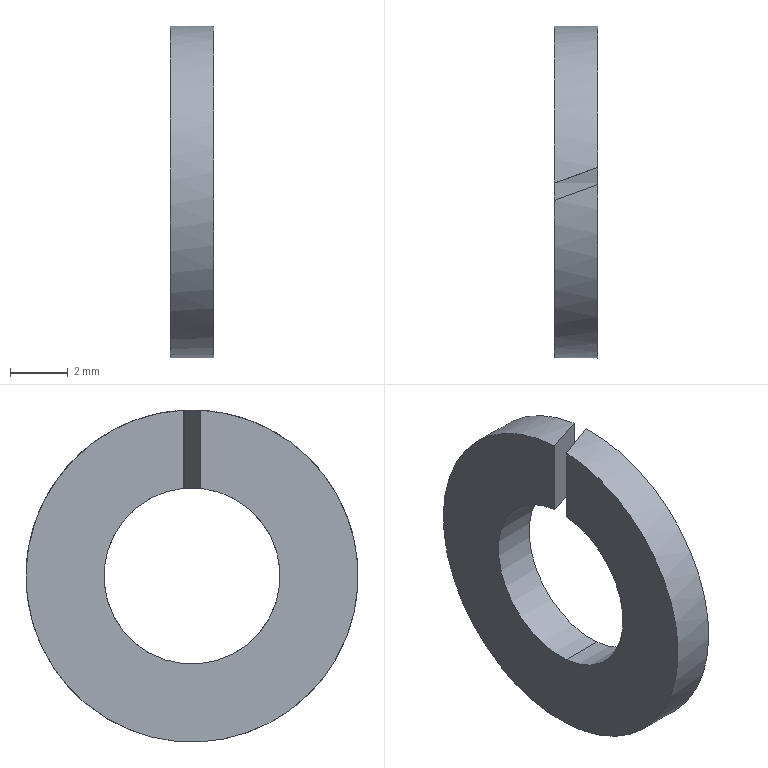Part | STEP file | KS B 1324 - No. 2 - 6 | 1 solid | 8 faces | box 1.5 x 11.5 x 11.5 mm | volume 109.527 mm3 | cylinder 4 | plane 4 | commonest cylinder face diameters 6.1 x2 11.5 x2
STEP:
#1=CARTESIAN_POINT('',(0.,0.,0.));
#2=DIRECTION('',(0.,0.,1.));
#3=DIRECTION('',(1.,0.,0.));
#4=AXIS2_PLACEMENT_3D('',#1,#2,#3);
#5=CARTESIAN_POINT('',(1.5,0.846,2.93));
#6=VERTEX_POINT('',#5);
#7=CARTESIAN_POINT('',(0.,0.3,3.035));
#8=VERTEX_POINT('',#7);
#9=CARTESIAN_POINT('',(1.5,0.846,2.93));
#10=CARTESIAN_POINT('',(1.009,0.6674,2.982));
#11=CARTESIAN_POINT('',(0.5081,0.4849,3.017));
#12=CARTESIAN_POINT('',(0.,0.3,3.035));
#13=(BOUNDED_CURVE()B_SPLINE_CURVE(3,(#9,#10,#11,#12),.UNSPECIFIED.,.F.,.F.)B_SPLINE_CURVE_WITH_KNOTS((4,4),(4.431,4.614),.PIECEWISE_BEZIER_KNOTS.)CURVE()GEOMETRIC_REPRESENTATION_ITEM()RATIONAL_B_SPLINE_CURVE((1.,0.9972,0.9972,1.))REPRESENTATION_ITEM(''));
#14=CARTESIAN_POINT('',(0.,0.,0.));
#15=DIRECTION('',(1.,0.,0.));
#16=DIRECTION('',(0.,-0.0895,-0.996));
#17=AXIS2_PLACEMENT_3D('',#14,#15,#16);
#18=CYLINDRICAL_SURFACE('',#17,3.05);
#19=CARTESIAN_POINT('',(2.95,1.5));
#20=CARTESIAN_POINT('',(2.953,1.478));
#21=CARTESIAN_POINT('',(2.958,1.433));
#22=CARTESIAN_POINT('',(2.967,1.366));
#23=CARTESIAN_POINT('',(2.975,1.299));
#24=CARTESIAN_POINT('',(2.983,1.232));
#25=CARTESIAN_POINT('',(2.992,1.164));
#26=CARTESIAN_POINT('',(3.,1.097));
#27=CARTESIAN_POINT('',(3.008,1.029));
#28=CARTESIAN_POINT('',(3.017,0.9611));
#29=CARTESIAN_POINT('',(3.025,0.893));
#30=CARTESIAN_POINT('',(3.033,0.8249));
#31=CARTESIAN_POINT('',(3.041,0.7566));
#32=CARTESIAN_POINT('',(3.05,0.6882));
#33=CARTESIAN_POINT('',(3.058,0.6197));
#34=CARTESIAN_POINT('',(3.066,0.5512));
#35=CARTESIAN_POINT('',(3.075,0.4825));
#36=CARTESIAN_POINT('',(3.083,0.4138));
#37=CARTESIAN_POINT('',(3.091,0.3449));
#38=CARTESIAN_POINT('',(3.1,0.2761));
#39=CARTESIAN_POINT('',(3.108,0.2071));
#40=CARTESIAN_POINT('',(3.116,0.1381));
#41=CARTESIAN_POINT('',(3.124,0.06908));
#42=CARTESIAN_POINT('',(3.13,0.02303));
#43=CARTESIAN_POINT('',(3.133,0.));
#44=B_SPLINE_CURVE_WITH_KNOTS('',3,(#19,#20,#21,#22,#23,#24,#25,#26,#27,#28,#29,#30,#31,#32,#33,#34,#35,#36,#37,#38,#39,#40,#41,#42,#43),.UNSPECIFIED.,.F.,.F.,(4,1,1,1,1,1,1,1,1,1,1,1,1,1,1,1,1,1,1,1,1,1,4),(4.431,4.44,4.448,4.456,4.465,4.473,4.481,4.489,4.498,4.506,4.514,4.523,4.531,4.539,4.547,4.556,4.564,4.572,4.581,4.589,4.597,4.606,4.614),.QUASI_UNIFORM_KNOTS.);
#45=(GEOMETRIC_REPRESENTATION_CONTEXT(2)PARAMETRIC_REPRESENTATION_CONTEXT()REPRESENTATION_CONTEXT('',''));
#46=DEFINITIONAL_REPRESENTATION('',(#44),#45);
#47=PCURVE('',#18,#46);
#48=CARTESIAN_POINT('',(0.,0.3,0.));
#49=DIRECTION('',(-0.342,0.9397,0.));
#50=DIRECTION('',(0.,0.,1.));
#51=AXIS2_PLACEMENT_3D('',#48,#49,#50);
#52=PLANE('',#51);
#53=CARTESIAN_POINT('',(2.93,1.596));
#54=CARTESIAN_POINT('',(2.982,1.074));
#55=CARTESIAN_POINT('',(3.017,0.5407));
#56=CARTESIAN_POINT('',(3.035,0.));
#57=(BOUNDED_CURVE()B_SPLINE_CURVE(3,(#53,#54,#55,#56),.UNSPECIFIED.,.F.,.F.)B_SPLINE_CURVE_WITH_KNOTS((4,4),(4.431,4.614),.PIECEWISE_BEZIER_KNOTS.)CURVE()GEOMETRIC_REPRESENTATION_ITEM()RATIONAL_B_SPLINE_CURVE((1.,0.9972,0.9972,1.))REPRESENTATION_ITEM(''));
#58=(GEOMETRIC_REPRESENTATION_CONTEXT(2)PARAMETRIC_REPRESENTATION_CONTEXT()REPRESENTATION_CONTEXT('',''));
#59=DEFINITIONAL_REPRESENTATION('',(#57),#58);
#60=PCURVE('',#52,#59);
#61=SURFACE_CURVE('',#13,(#47,#60),.PCURVE_S1.);
#62=EDGE_CURVE('',#6,#8,#61,.T.);
#63=ORIENTED_EDGE('',*,*,#62,.F.);
#64=CARTESIAN_POINT('',(1.5,-0.273,-3.038));
#65=VERTEX_POINT('',#64);
#66=CARTESIAN_POINT('',(1.5,0.,0.));
#67=DIRECTION('',(-1.,0.,0.));
#68=DIRECTION('',(0.,-1.,0.));
#69=AXIS2_PLACEMENT_3D('',#66,#67,#68);
#70=CIRCLE('',#69,3.05);
#71=CARTESIAN_POINT('',(4.802,1.5));
#72=DIRECTION('',(-1.,0.));
#73=VECTOR('',#72,1.);
#74=LINE('',#71,#73);
#75=(GEOMETRIC_REPRESENTATION_CONTEXT(2)PARAMETRIC_REPRESENTATION_CONTEXT()REPRESENTATION_CONTEXT('',''));
#76=DEFINITIONAL_REPRESENTATION('',(#74),#75);
#77=PCURVE('',#18,#76);
#78=CARTESIAN_POINT('',(1.5,0.,0.));
#79=DIRECTION('',(-1.,0.,0.));
#80=DIRECTION('',(0.,0.,1.));
#81=AXIS2_PLACEMENT_3D('',#78,#79,#80);
#82=PLANE('',#81);
#83=CARTESIAN_POINT('',(0.,0.));
#84=DIRECTION('',(0.,-1.));
#85=AXIS2_PLACEMENT_2D('',#83,#84);
#86=CIRCLE('',#85,3.05);
#87=(GEOMETRIC_REPRESENTATION_CONTEXT(2)PARAMETRIC_REPRESENTATION_CONTEXT()REPRESENTATION_CONTEXT('',''));
#88=DEFINITIONAL_REPRESENTATION('',(#86),#87);
#89=PCURVE('',#82,#88);
#90=SURFACE_CURVE('',#70,(#77,#89),.PCURVE_S1.);
#91=EDGE_CURVE('',#6,#65,#90,.T.);
#92=ORIENTED_EDGE('',*,*,#91,.T.);
#93=CARTESIAN_POINT('',(0.,-0.273,-3.038));
#94=VERTEX_POINT('',#93);
#95=CARTESIAN_POINT('',(0.,-0.273,-3.038));
#96=DIRECTION('',(1.,0.,0.));
#97=VECTOR('',#96,1.);
#98=LINE('',#95,#97);
#99=CARTESIAN_POINT('',(0.,0.));
#100=DIRECTION('',(0.,1.));
#101=VECTOR('',#100,1.);
#102=LINE('',#99,#101);
#103=(GEOMETRIC_REPRESENTATION_CONTEXT(2)PARAMETRIC_REPRESENTATION_CONTEXT()REPRESENTATION_CONTEXT('',''));
#104=DEFINITIONAL_REPRESENTATION('',(#102),#103);
#105=PCURVE('',#18,#104);
#106=CARTESIAN_POINT('',(0.,0.,0.));
#107=DIRECTION('',(1.,0.,0.));
#108=DIRECTION('',(0.,-0.0895,-0.996));
#109=AXIS2_PLACEMENT_3D('',#106,#107,#108);
#110=CYLINDRICAL_SURFACE('',#109,3.05);
#111=CARTESIAN_POINT('',(6.283,0.));
#112=DIRECTION('',(0.,1.));
#113=VECTOR('',#112,1.);
#114=LINE('',#111,#113);
#115=(GEOMETRIC_REPRESENTATION_CONTEXT(2)PARAMETRIC_REPRESENTATION_CONTEXT()REPRESENTATION_CONTEXT('',''));
#116=DEFINITIONAL_REPRESENTATION('',(#114),#115);
#117=PCURVE('',#110,#116);
#118=SURFACE_CURVE('',#98,(#105,#117),.PCURVE_S1.);
#119=EDGE_CURVE('',#94,#65,#118,.T.);
#120=ORIENTED_EDGE('',*,*,#119,.F.);
#121=CARTESIAN_POINT('',(0.,0.,0.));
#122=DIRECTION('',(1.,0.,0.));
#123=DIRECTION('',(0.,-1.,0.));
#124=AXIS2_PLACEMENT_3D('',#121,#122,#123);
#125=CIRCLE('',#124,3.05);
#126=CARTESIAN_POINT('',(-1.481,0.));
#127=DIRECTION('',(1.,0.));
#128=VECTOR('',#127,1.);
#129=LINE('',#126,#128);
#130=(GEOMETRIC_REPRESENTATION_CONTEXT(2)PARAMETRIC_REPRESENTATION_CONTEXT()REPRESENTATION_CONTEXT('',''));
#131=DEFINITIONAL_REPRESENTATION('',(#129),#130);
#132=PCURVE('',#18,#131);
#133=CARTESIAN_POINT('',(0.,0.,0.));
#134=DIRECTION('',(-1.,0.,0.));
#135=DIRECTION('',(0.,0.,1.));
#136=AXIS2_PLACEMENT_3D('',#133,#134,#135);
#137=PLANE('',#136);
#138=CARTESIAN_POINT('',(0.,-3.05));
#139=CARTESIAN_POINT('',(-5.283,-3.05));
#140=CARTESIAN_POINT('',(-2.641,1.525));
#141=CARTESIAN_POINT('',(0.,6.1));
#142=CARTESIAN_POINT('',(2.641,1.525));
#143=CARTESIAN_POINT('',(5.283,-3.05));
#144=CARTESIAN_POINT('',(0.,-3.05));
#145=(BOUNDED_CURVE()B_SPLINE_CURVE(2,(#138,#139,#140,#141,#142,#143,#144),.UNSPECIFIED.,.T.,.F.)B_SPLINE_CURVE_WITH_KNOTS((1,2,2,2,2,1),(-2.094,0.,2.094,4.189,6.283,8.378),.UNSPECIFIED.)CURVE()GEOMETRIC_REPRESENTATION_ITEM()RATIONAL_B_SPLINE_CURVE((1.,0.5,1.,0.5,1.,0.5,1.))REPRESENTATION_ITEM(''));
#146=(GEOMETRIC_REPRESENTATION_CONTEXT(2)PARAMETRIC_REPRESENTATION_CONTEXT()REPRESENTATION_CONTEXT('',''));
#147=DEFINITIONAL_REPRESENTATION('',(#145),#146);
#148=PCURVE('',#137,#147);
#149=SURFACE_CURVE('',#125,(#132,#148),.PCURVE_S1.);
#150=EDGE_CURVE('',#94,#8,#149,.T.);
#151=ORIENTED_EDGE('',*,*,#150,.T.);
#152=EDGE_LOOP('',(#63,#92,#120,#151));
#153=FACE_BOUND('',#152,.F.);
#154=ADVANCED_FACE('',(#153),#18,.F.);
#155=CARTESIAN_POINT('',(0.,-0.273,-5.744));
#156=VERTEX_POINT('',#155);
#157=CARTESIAN_POINT('',(0.,-0.3,5.742));
#158=VERTEX_POINT('',#157);
#159=CARTESIAN_POINT('',(0.,0.,0.));
#160=DIRECTION('',(-1.,0.,0.));
#161=DIRECTION('',(0.,-1.,0.));
#162=AXIS2_PLACEMENT_3D('',#159,#160,#161);
#163=CIRCLE('',#162,5.75);
#164=CARTESIAN_POINT('',(0.,0.,0.));
#165=DIRECTION('',(1.,0.,0.));
#166=DIRECTION('',(0.,-0.04747,-0.9989));
#167=AXIS2_PLACEMENT_3D('',#164,#165,#166);
#168=CYLINDRICAL_SURFACE('',#167,5.75);
#169=CARTESIAN_POINT('',(11.043,0.));
#170=DIRECTION('',(-1.,0.));
#171=VECTOR('',#170,1.);
#172=LINE('',#169,#171);
#173=(GEOMETRIC_REPRESENTATION_CONTEXT(2)PARAMETRIC_REPRESENTATION_CONTEXT()REPRESENTATION_CONTEXT('',''));
#174=DEFINITIONAL_REPRESENTATION('',(#172),#173);
#175=PCURVE('',#168,#174);
#176=CARTESIAN_POINT('',(0.,0.));
#177=DIRECTION('',(0.,-1.));
#178=AXIS2_PLACEMENT_2D('',#176,#177);
#179=CIRCLE('',#178,5.75);
#180=(GEOMETRIC_REPRESENTATION_CONTEXT(2)PARAMETRIC_REPRESENTATION_CONTEXT()REPRESENTATION_CONTEXT('',''));
#181=DEFINITIONAL_REPRESENTATION('',(#179),#180);
#182=PCURVE('',#137,#181);
#183=SURFACE_CURVE('',#163,(#175,#182),.PCURVE_S1.);
#184=EDGE_CURVE('',#156,#158,#183,.T.);
#185=ORIENTED_EDGE('',*,*,#184,.F.);
#186=CARTESIAN_POINT('',(1.5,-0.273,-5.744));
#187=VERTEX_POINT('',#186);
#188=CARTESIAN_POINT('',(0.,-0.273,-5.744));
#189=DIRECTION('',(1.,0.,0.));
#190=VECTOR('',#189,1.);
#191=LINE('',#188,#190);
#192=CARTESIAN_POINT('',(6.283,0.));
#193=DIRECTION('',(0.,1.));
#194=VECTOR('',#193,1.);
#195=LINE('',#192,#194);
#196=(GEOMETRIC_REPRESENTATION_CONTEXT(2)PARAMETRIC_REPRESENTATION_CONTEXT()REPRESENTATION_CONTEXT('',''));
#197=DEFINITIONAL_REPRESENTATION('',(#195),#196);
#198=PCURVE('',#168,#197);
#199=CARTESIAN_POINT('',(0.,0.,0.));
#200=DIRECTION('',(1.,0.,0.));
#201=DIRECTION('',(0.,-0.04747,-0.9989));
#202=AXIS2_PLACEMENT_3D('',#199,#200,#201);
#203=CYLINDRICAL_SURFACE('',#202,5.75);
#204=CARTESIAN_POINT('',(0.,0.));
#205=DIRECTION('',(0.,1.));
#206=VECTOR('',#205,1.);
#207=LINE('',#204,#206);
#208=(GEOMETRIC_REPRESENTATION_CONTEXT(2)PARAMETRIC_REPRESENTATION_CONTEXT()REPRESENTATION_CONTEXT('',''));
#209=DEFINITIONAL_REPRESENTATION('',(#207),#208);
#210=PCURVE('',#203,#209);
#211=SURFACE_CURVE('',#191,(#198,#210),.PCURVE_S1.);
#212=EDGE_CURVE('',#156,#187,#211,.T.);
#213=ORIENTED_EDGE('',*,*,#212,.T.);
#214=CARTESIAN_POINT('',(1.5,0.246,5.745));
#215=VERTEX_POINT('',#214);
#216=CARTESIAN_POINT('',(1.5,0.,0.));
#217=DIRECTION('',(-1.,0.,0.));
#218=DIRECTION('',(0.,-1.,0.));
#219=AXIS2_PLACEMENT_3D('',#216,#217,#218);
#220=CIRCLE('',#219,5.75);
#221=CARTESIAN_POINT('',(11.043,1.5));
#222=DIRECTION('',(-1.,0.));
#223=VECTOR('',#222,1.);
#224=LINE('',#221,#223);
#225=(GEOMETRIC_REPRESENTATION_CONTEXT(2)PARAMETRIC_REPRESENTATION_CONTEXT()REPRESENTATION_CONTEXT('',''));
#226=DEFINITIONAL_REPRESENTATION('',(#224),#225);
#227=PCURVE('',#168,#226);
#228=CARTESIAN_POINT('',(0.,0.));
#229=DIRECTION('',(0.,-1.));
#230=AXIS2_PLACEMENT_2D('',#228,#229);
#231=CIRCLE('',#230,5.75);
#232=(GEOMETRIC_REPRESENTATION_CONTEXT(2)PARAMETRIC_REPRESENTATION_CONTEXT()REPRESENTATION_CONTEXT('',''));
#233=DEFINITIONAL_REPRESENTATION('',(#231),#232);
#234=PCURVE('',#82,#233);
#235=SURFACE_CURVE('',#220,(#227,#234),.PCURVE_S1.);
#236=EDGE_CURVE('',#187,#215,#235,.T.);
#237=ORIENTED_EDGE('',*,*,#236,.T.);
#238=CARTESIAN_POINT('',(1.5,0.246,5.745));
#239=CARTESIAN_POINT('',(1.,0.064,5.753));
#240=CARTESIAN_POINT('',(0.4997,-0.1181,5.752));
#241=CARTESIAN_POINT('',(0.,-0.3,5.742));
#242=(BOUNDED_CURVE()B_SPLINE_CURVE(3,(#238,#239,#240,#241),.UNSPECIFIED.,.F.,.F.)B_SPLINE_CURVE_WITH_KNOTS((4,4),(4.67,4.765),.PIECEWISE_BEZIER_KNOTS.)CURVE()GEOMETRIC_REPRESENTATION_ITEM()RATIONAL_B_SPLINE_CURVE((1.,0.9992,0.9992,1.))REPRESENTATION_ITEM(''));
#243=CARTESIAN_POINT('',(3.146,1.5));
#244=CARTESIAN_POINT('',(3.148,1.477));
#245=CARTESIAN_POINT('',(3.151,1.432));
#246=CARTESIAN_POINT('',(3.155,1.364));
#247=CARTESIAN_POINT('',(3.159,1.296));
#248=CARTESIAN_POINT('',(3.164,1.227));
#249=CARTESIAN_POINT('',(3.168,1.159));
#250=CARTESIAN_POINT('',(3.172,1.091));
#251=CARTESIAN_POINT('',(3.177,1.023));
#252=CARTESIAN_POINT('',(3.181,0.9546));
#253=CARTESIAN_POINT('',(3.185,0.8864));
#254=CARTESIAN_POINT('',(3.189,0.8181));
#255=CARTESIAN_POINT('',(3.194,0.7499));
#256=CARTESIAN_POINT('',(3.198,0.6817));
#257=CARTESIAN_POINT('',(3.202,0.6135));
#258=CARTESIAN_POINT('',(3.207,0.5453));
#259=CARTESIAN_POINT('',(3.211,0.4771));
#260=CARTESIAN_POINT('',(3.215,0.4089));
#261=CARTESIAN_POINT('',(3.22,0.3407));
#262=CARTESIAN_POINT('',(3.224,0.2725));
#263=CARTESIAN_POINT('',(3.228,0.2044));
#264=CARTESIAN_POINT('',(3.233,0.1362));
#265=CARTESIAN_POINT('',(3.237,0.0681));
#266=CARTESIAN_POINT('',(3.24,0.0227));
#267=CARTESIAN_POINT('',(3.241,0.));
#268=B_SPLINE_CURVE_WITH_KNOTS('',3,(#243,#244,#245,#246,#247,#248,#249,#250,#251,#252,#253,#254,#255,#256,#257,#258,#259,#260,#261,#262,#263,#264,#265,#266,#267),.UNSPECIFIED.,.F.,.F.,(4,1,1,1,1,1,1,1,1,1,1,1,1,1,1,1,1,1,1,1,1,1,4),(4.67,4.674,4.678,4.683,4.687,4.691,4.696,4.7,4.704,4.708,4.713,4.717,4.721,4.726,4.73,4.734,4.739,4.743,4.747,4.752,4.756,4.76,4.765),.QUASI_UNIFORM_KNOTS.);
#269=(GEOMETRIC_REPRESENTATION_CONTEXT(2)PARAMETRIC_REPRESENTATION_CONTEXT()REPRESENTATION_CONTEXT('',''));
#270=DEFINITIONAL_REPRESENTATION('',(#268),#269);
#271=PCURVE('',#168,#270);
#272=CARTESIAN_POINT('',(1.5,0.246,0.));
#273=DIRECTION('',(0.342,-0.9397,0.));
#274=DIRECTION('',(0.,0.,-1.));
#275=AXIS2_PLACEMENT_3D('',#272,#273,#274);
#276=PLANE('',#275);
#277=CARTESIAN_POINT('',(-5.745,0.));
#278=CARTESIAN_POINT('',(-5.753,-0.532));
#279=CARTESIAN_POINT('',(-5.752,-1.064));
#280=CARTESIAN_POINT('',(-5.742,-1.596));
#281=(BOUNDED_CURVE()B_SPLINE_CURVE(3,(#277,#278,#279,#280),.UNSPECIFIED.,.F.,.F.)B_SPLINE_CURVE_WITH_KNOTS((4,4),(4.67,4.765),.PIECEWISE_BEZIER_KNOTS.)CURVE()GEOMETRIC_REPRESENTATION_ITEM()RATIONAL_B_SPLINE_CURVE((1.,0.9992,0.9992,1.))REPRESENTATION_ITEM(''));
#282=(GEOMETRIC_REPRESENTATION_CONTEXT(2)PARAMETRIC_REPRESENTATION_CONTEXT()REPRESENTATION_CONTEXT('',''));
#283=DEFINITIONAL_REPRESENTATION('',(#281),#282);
#284=PCURVE('',#276,#283);
#285=SURFACE_CURVE('',#242,(#271,#284),.PCURVE_S1.);
#286=EDGE_CURVE('',#215,#158,#285,.T.);
#287=ORIENTED_EDGE('',*,*,#286,.T.);
#288=EDGE_LOOP('',(#185,#213,#237,#287));
#289=FACE_BOUND('',#288,.T.);
#290=ADVANCED_FACE('',(#289),#168,.T.);
#291=CARTESIAN_POINT('',(0.,-0.3,3.035));
#292=VERTEX_POINT('',#291);
#293=CARTESIAN_POINT('',(0.,-0.3,0.));
#294=DIRECTION('',(0.,0.,-1.));
#295=VECTOR('',#294,1.);
#296=LINE('',#293,#295);
#297=CARTESIAN_POINT('',(0.,-0.3));
#298=DIRECTION('',(-1.,0.));
#299=VECTOR('',#298,1.);
#300=LINE('',#297,#299);
#301=(GEOMETRIC_REPRESENTATION_CONTEXT(2)PARAMETRIC_REPRESENTATION_CONTEXT()REPRESENTATION_CONTEXT('',''));
#302=DEFINITIONAL_REPRESENTATION('',(#300),#301);
#303=PCURVE('',#137,#302);
#304=CARTESIAN_POINT('',(0.,-1.596));
#305=DIRECTION('',(1.,0.));
#306=VECTOR('',#305,1.);
#307=LINE('',#304,#306);
#308=(GEOMETRIC_REPRESENTATION_CONTEXT(2)PARAMETRIC_REPRESENTATION_CONTEXT()REPRESENTATION_CONTEXT('',''));
#309=DEFINITIONAL_REPRESENTATION('',(#307),#308);
#310=PCURVE('',#276,#309);
#311=SURFACE_CURVE('',#296,(#303,#310),.PCURVE_S1.);
#312=EDGE_CURVE('',#158,#292,#311,.T.);
#313=ORIENTED_EDGE('',*,*,#312,.T.);
#314=CARTESIAN_POINT('',(0.,0.,0.));
#315=DIRECTION('',(1.,0.,0.));
#316=DIRECTION('',(0.,-1.,0.));
#317=AXIS2_PLACEMENT_3D('',#314,#315,#316);
#318=CIRCLE('',#317,3.05);
#319=CARTESIAN_POINT('',(0.,-3.05));
#320=CARTESIAN_POINT('',(-5.283,-3.05));
#321=CARTESIAN_POINT('',(-2.641,1.525));
#322=CARTESIAN_POINT('',(0.,6.1));
#323=CARTESIAN_POINT('',(2.641,1.525));
#324=CARTESIAN_POINT('',(5.283,-3.05));
#325=CARTESIAN_POINT('',(0.,-3.05));
#326=(BOUNDED_CURVE()B_SPLINE_CURVE(2,(#319,#320,#321,#322,#323,#324,#325),.UNSPECIFIED.,.T.,.F.)B_SPLINE_CURVE_WITH_KNOTS((1,2,2,2,2,1),(-2.094,0.,2.094,4.189,6.283,8.378),.UNSPECIFIED.)CURVE()GEOMETRIC_REPRESENTATION_ITEM()RATIONAL_B_SPLINE_CURVE((1.,0.5,1.,0.5,1.,0.5,1.))REPRESENTATION_ITEM(''));
#327=(GEOMETRIC_REPRESENTATION_CONTEXT(2)PARAMETRIC_REPRESENTATION_CONTEXT()REPRESENTATION_CONTEXT('',''));
#328=DEFINITIONAL_REPRESENTATION('',(#326),#327);
#329=PCURVE('',#137,#328);
#330=CARTESIAN_POINT('',(-1.481,0.));
#331=DIRECTION('',(1.,0.));
#332=VECTOR('',#331,1.);
#333=LINE('',#330,#332);
#334=(GEOMETRIC_REPRESENTATION_CONTEXT(2)PARAMETRIC_REPRESENTATION_CONTEXT()REPRESENTATION_CONTEXT('',''));
#335=DEFINITIONAL_REPRESENTATION('',(#333),#334);
#336=PCURVE('',#110,#335);
#337=SURFACE_CURVE('',#318,(#329,#336),.PCURVE_S1.);
#338=EDGE_CURVE('',#292,#94,#337,.T.);
#339=ORIENTED_EDGE('',*,*,#338,.T.);
#340=ORIENTED_EDGE('',*,*,#150,.T.);
#341=CARTESIAN_POINT('',(0.,0.3,5.742));
#342=VERTEX_POINT('',#341);
#343=CARTESIAN_POINT('',(0.,0.3,0.));
#344=DIRECTION('',(0.,0.,1.));
#345=VECTOR('',#344,1.);
#346=LINE('',#343,#345);
#347=CARTESIAN_POINT('',(0.,0.3));
#348=DIRECTION('',(1.,0.));
#349=VECTOR('',#348,1.);
#350=LINE('',#347,#349);
#351=(GEOMETRIC_REPRESENTATION_CONTEXT(2)PARAMETRIC_REPRESENTATION_CONTEXT()REPRESENTATION_CONTEXT('',''));
#352=DEFINITIONAL_REPRESENTATION('',(#350),#351);
#353=PCURVE('',#137,#352);
#354=CARTESIAN_POINT('',(0.,0.));
#355=DIRECTION('',(1.,0.));
#356=VECTOR('',#355,1.);
#357=LINE('',#354,#356);
#358=(GEOMETRIC_REPRESENTATION_CONTEXT(2)PARAMETRIC_REPRESENTATION_CONTEXT()REPRESENTATION_CONTEXT('',''));
#359=DEFINITIONAL_REPRESENTATION('',(#357),#358);
#360=PCURVE('',#52,#359);
#361=SURFACE_CURVE('',#346,(#353,#360),.PCURVE_S1.);
#362=EDGE_CURVE('',#8,#342,#361,.T.);
#363=ORIENTED_EDGE('',*,*,#362,.T.);
#364=CARTESIAN_POINT('',(0.,0.,0.));
#365=DIRECTION('',(-1.,0.,0.));
#366=DIRECTION('',(0.,-1.,0.));
#367=AXIS2_PLACEMENT_3D('',#364,#365,#366);
#368=CIRCLE('',#367,5.75);
#369=CARTESIAN_POINT('',(0.,0.));
#370=DIRECTION('',(0.,-1.));
#371=AXIS2_PLACEMENT_2D('',#369,#370);
#372=CIRCLE('',#371,5.75);
#373=(GEOMETRIC_REPRESENTATION_CONTEXT(2)PARAMETRIC_REPRESENTATION_CONTEXT()REPRESENTATION_CONTEXT('',''));
#374=DEFINITIONAL_REPRESENTATION('',(#372),#373);
#375=PCURVE('',#137,#374);
#376=CARTESIAN_POINT('',(4.76,0.));
#377=DIRECTION('',(-1.,0.));
#378=VECTOR('',#377,1.);
#379=LINE('',#376,#378);
#380=(GEOMETRIC_REPRESENTATION_CONTEXT(2)PARAMETRIC_REPRESENTATION_CONTEXT()REPRESENTATION_CONTEXT('',''));
#381=DEFINITIONAL_REPRESENTATION('',(#379),#380);
#382=PCURVE('',#203,#381);
#383=SURFACE_CURVE('',#368,(#375,#382),.PCURVE_S1.);
#384=EDGE_CURVE('',#342,#156,#383,.T.);
#385=ORIENTED_EDGE('',*,*,#384,.T.);
#386=ORIENTED_EDGE('',*,*,#184,.T.);
#387=EDGE_LOOP('',(#313,#339,#340,#363,#385,#386));
#388=FACE_BOUND('',#387,.T.);
#389=ADVANCED_FACE('',(#388),#137,.T.);
#390=ORIENTED_EDGE('',*,*,#212,.F.);
#391=ORIENTED_EDGE('',*,*,#384,.F.);
#392=CARTESIAN_POINT('',(1.5,0.846,5.687));
#393=VERTEX_POINT('',#392);
#394=CARTESIAN_POINT('',(0.,0.3,5.742));
#395=CARTESIAN_POINT('',(0.5022,0.4828,5.733));
#396=CARTESIAN_POINT('',(1.003,0.6649,5.714));
#397=CARTESIAN_POINT('',(1.5,0.846,5.687));
#398=(BOUNDED_CURVE()B_SPLINE_CURVE(3,(#394,#395,#396,#397),.UNSPECIFIED.,.F.,.F.)B_SPLINE_CURVE_WITH_KNOTS((4,4),(1.623,1.718),.PIECEWISE_BEZIER_KNOTS.)CURVE()GEOMETRIC_REPRESENTATION_ITEM()RATIONAL_B_SPLINE_CURVE((1.,0.9992,0.9992,1.))REPRESENTATION_ITEM(''));
#399=CARTESIAN_POINT('',(3.137,0.));
#400=CARTESIAN_POINT('',(3.135,0.02281));
#401=CARTESIAN_POINT('',(3.133,0.06843));
#402=CARTESIAN_POINT('',(3.128,0.1368));
#403=CARTESIAN_POINT('',(3.124,0.2052));
#404=CARTESIAN_POINT('',(3.12,0.2736));
#405=CARTESIAN_POINT('',(3.115,0.342));
#406=CARTESIAN_POINT('',(3.111,0.4104));
#407=CARTESIAN_POINT('',(3.107,0.4787));
#408=CARTESIAN_POINT('',(3.102,0.547));
#409=CARTESIAN_POINT('',(3.098,0.6153));
#410=CARTESIAN_POINT('',(3.093,0.6836));
#411=CARTESIAN_POINT('',(3.089,0.7518));
#412=CARTESIAN_POINT('',(3.085,0.82));
#413=CARTESIAN_POINT('',(3.08,0.8882));
#414=CARTESIAN_POINT('',(3.076,0.9563));
#415=CARTESIAN_POINT('',(3.072,1.024));
#416=CARTESIAN_POINT('',(3.067,1.092));
#417=CARTESIAN_POINT('',(3.063,1.161));
#418=CARTESIAN_POINT('',(3.059,1.229));
#419=CARTESIAN_POINT('',(3.054,1.296));
#420=CARTESIAN_POINT('',(3.05,1.364));
#421=CARTESIAN_POINT('',(3.046,1.432));
#422=CARTESIAN_POINT('',(3.043,1.477));
#423=CARTESIAN_POINT('',(3.041,1.5));
#424=B_SPLINE_CURVE_WITH_KNOTS('',3,(#399,#400,#401,#402,#403,#404,#405,#406,#407,#408,#409,#410,#411,#412,#413,#414,#415,#416,#417,#418,#419,#420,#421,#422,#423),.UNSPECIFIED.,.F.,.F.,(4,1,1,1,1,1,1,1,1,1,1,1,1,1,1,1,1,1,1,1,1,1,4),(1.623,1.627,1.632,1.636,1.64,1.645,1.649,1.653,1.658,1.662,1.666,1.671,1.675,1.679,1.684,1.688,1.692,1.697,1.701,1.705,1.71,1.714,1.718),.QUASI_UNIFORM_KNOTS.);
#425=(GEOMETRIC_REPRESENTATION_CONTEXT(2)PARAMETRIC_REPRESENTATION_CONTEXT()REPRESENTATION_CONTEXT('',''));
#426=DEFINITIONAL_REPRESENTATION('',(#424),#425);
#427=PCURVE('',#203,#426);
#428=CARTESIAN_POINT('',(5.742,0.));
#429=CARTESIAN_POINT('',(5.733,0.5344));
#430=CARTESIAN_POINT('',(5.714,1.067));
#431=CARTESIAN_POINT('',(5.687,1.596));
#432=(BOUNDED_CURVE()B_SPLINE_CURVE(3,(#428,#429,#430,#431),.UNSPECIFIED.,.F.,.F.)B_SPLINE_CURVE_WITH_KNOTS((4,4),(1.623,1.718),.PIECEWISE_BEZIER_KNOTS.)CURVE()GEOMETRIC_REPRESENTATION_ITEM()RATIONAL_B_SPLINE_CURVE((1.,0.9992,0.9992,1.))REPRESENTATION_ITEM(''));
#433=(GEOMETRIC_REPRESENTATION_CONTEXT(2)PARAMETRIC_REPRESENTATION_CONTEXT()REPRESENTATION_CONTEXT('',''));
#434=DEFINITIONAL_REPRESENTATION('',(#432),#433);
#435=PCURVE('',#52,#434);
#436=SURFACE_CURVE('',#398,(#427,#435),.PCURVE_S1.);
#437=EDGE_CURVE('',#342,#393,#436,.T.);
#438=ORIENTED_EDGE('',*,*,#437,.T.);
#439=CARTESIAN_POINT('',(1.5,0.,0.));
#440=DIRECTION('',(-1.,0.,0.));
#441=DIRECTION('',(0.,-1.,0.));
#442=AXIS2_PLACEMENT_3D('',#439,#440,#441);
#443=CIRCLE('',#442,5.75);
#444=CARTESIAN_POINT('',(4.76,1.5));
#445=DIRECTION('',(-1.,0.));
#446=VECTOR('',#445,1.);
#447=LINE('',#444,#446);
#448=(GEOMETRIC_REPRESENTATION_CONTEXT(2)PARAMETRIC_REPRESENTATION_CONTEXT()REPRESENTATION_CONTEXT('',''));
#449=DEFINITIONAL_REPRESENTATION('',(#447),#448);
#450=PCURVE('',#203,#449);
#451=CARTESIAN_POINT('',(0.,0.));
#452=DIRECTION('',(0.,-1.));
#453=AXIS2_PLACEMENT_2D('',#451,#452);
#454=CIRCLE('',#453,5.75);
#455=(GEOMETRIC_REPRESENTATION_CONTEXT(2)PARAMETRIC_REPRESENTATION_CONTEXT()REPRESENTATION_CONTEXT('',''));
#456=DEFINITIONAL_REPRESENTATION('',(#454),#455);
#457=PCURVE('',#82,#456);
#458=SURFACE_CURVE('',#443,(#450,#457),.PCURVE_S1.);
#459=EDGE_CURVE('',#393,#187,#458,.T.);
#460=ORIENTED_EDGE('',*,*,#459,.T.);
#461=EDGE_LOOP('',(#390,#391,#438,#460));
#462=FACE_BOUND('',#461,.T.);
#463=ADVANCED_FACE('',(#462),#203,.T.);
#464=CARTESIAN_POINT('',(1.5,0.246,3.04));
#465=VERTEX_POINT('',#464);
#466=CARTESIAN_POINT('',(1.5,0.,0.));
#467=DIRECTION('',(-1.,0.,0.));
#468=DIRECTION('',(0.,-1.,0.));
#469=AXIS2_PLACEMENT_3D('',#466,#467,#468);
#470=CIRCLE('',#469,3.05);
#471=CARTESIAN_POINT('',(11.085,1.5));
#472=DIRECTION('',(-1.,0.));
#473=VECTOR('',#472,1.);
#474=LINE('',#471,#473);
#475=(GEOMETRIC_REPRESENTATION_CONTEXT(2)PARAMETRIC_REPRESENTATION_CONTEXT()REPRESENTATION_CONTEXT('',''));
#476=DEFINITIONAL_REPRESENTATION('',(#474),#475);
#477=PCURVE('',#110,#476);
#478=CARTESIAN_POINT('',(0.,0.));
#479=DIRECTION('',(0.,-1.));
#480=AXIS2_PLACEMENT_2D('',#478,#479);
#481=CIRCLE('',#480,3.05);
#482=(GEOMETRIC_REPRESENTATION_CONTEXT(2)PARAMETRIC_REPRESENTATION_CONTEXT()REPRESENTATION_CONTEXT('',''));
#483=DEFINITIONAL_REPRESENTATION('',(#481),#482);
#484=PCURVE('',#82,#483);
#485=SURFACE_CURVE('',#470,(#477,#484),.PCURVE_S1.);
#486=EDGE_CURVE('',#65,#465,#485,.T.);
#487=ORIENTED_EDGE('',*,*,#486,.T.);
#488=CARTESIAN_POINT('',(0.,-0.3,3.035));
#489=CARTESIAN_POINT('',(0.4989,-0.1184,3.053));
#490=CARTESIAN_POINT('',(1.,0.06407,3.055));
#491=CARTESIAN_POINT('',(1.5,0.246,3.04));
#492=(BOUNDED_CURVE()B_SPLINE_CURVE(3,(#488,#489,#490,#491),.UNSPECIFIED.,.F.,.F.)B_SPLINE_CURVE_WITH_KNOTS((4,4),(1.472,1.652),.PIECEWISE_BEZIER_KNOTS.)CURVE()GEOMETRIC_REPRESENTATION_ITEM()RATIONAL_B_SPLINE_CURVE((1.,0.9973,0.9973,1.))REPRESENTATION_ITEM(''));
#493=CARTESIAN_POINT('',(3.33,0.));
#494=CARTESIAN_POINT('',(3.327,0.02262));
#495=CARTESIAN_POINT('',(3.322,0.06788));
#496=CARTESIAN_POINT('',(3.313,0.1358));
#497=CARTESIAN_POINT('',(3.305,0.2039));
#498=CARTESIAN_POINT('',(3.297,0.272));
#499=CARTESIAN_POINT('',(3.289,0.3401));
#500=CARTESIAN_POINT('',(3.281,0.4083));
#501=CARTESIAN_POINT('',(3.273,0.4765));
#502=CARTESIAN_POINT('',(3.265,0.5448));
#503=CARTESIAN_POINT('',(3.256,0.6131));
#504=CARTESIAN_POINT('',(3.248,0.6814));
#505=CARTESIAN_POINT('',(3.24,0.7497));
#506=CARTESIAN_POINT('',(3.232,0.818));
#507=CARTESIAN_POINT('',(3.224,0.8863));
#508=CARTESIAN_POINT('',(3.216,0.9547));
#509=CARTESIAN_POINT('',(3.208,1.023));
#510=CARTESIAN_POINT('',(3.199,1.091));
#511=CARTESIAN_POINT('',(3.191,1.159));
#512=CARTESIAN_POINT('',(3.183,1.228));
#513=CARTESIAN_POINT('',(3.175,1.296));
#514=CARTESIAN_POINT('',(3.167,1.364));
#515=CARTESIAN_POINT('',(3.159,1.432));
#516=CARTESIAN_POINT('',(3.153,1.477));
#517=CARTESIAN_POINT('',(3.15,1.5));
#518=B_SPLINE_CURVE_WITH_KNOTS('',3,(#493,#494,#495,#496,#497,#498,#499,#500,#501,#502,#503,#504,#505,#506,#507,#508,#509,#510,#511,#512,#513,#514,#515,#516,#517),.UNSPECIFIED.,.F.,.F.,(4,1,1,1,1,1,1,1,1,1,1,1,1,1,1,1,1,1,1,1,1,1,4),(1.472,1.48,1.489,1.497,1.505,1.513,1.521,1.529,1.537,1.546,1.554,1.562,1.57,1.578,1.586,1.594,1.603,1.611,1.619,1.627,1.635,1.643,1.652),.QUASI_UNIFORM_KNOTS.);
#519=(GEOMETRIC_REPRESENTATION_CONTEXT(2)PARAMETRIC_REPRESENTATION_CONTEXT()REPRESENTATION_CONTEXT('',''));
#520=DEFINITIONAL_REPRESENTATION('',(#518),#519);
#521=PCURVE('',#110,#520);
#522=CARTESIAN_POINT('',(-3.035,-1.596));
#523=CARTESIAN_POINT('',(-3.053,-1.065));
#524=CARTESIAN_POINT('',(-3.055,-0.5318));
#525=CARTESIAN_POINT('',(-3.04,0.));
#526=(BOUNDED_CURVE()B_SPLINE_CURVE(3,(#522,#523,#524,#525),.UNSPECIFIED.,.F.,.F.)B_SPLINE_CURVE_WITH_KNOTS((4,4),(1.472,1.652),.PIECEWISE_BEZIER_KNOTS.)CURVE()GEOMETRIC_REPRESENTATION_ITEM()RATIONAL_B_SPLINE_CURVE((1.,0.9973,0.9973,1.))REPRESENTATION_ITEM(''));
#527=(GEOMETRIC_REPRESENTATION_CONTEXT(2)PARAMETRIC_REPRESENTATION_CONTEXT()REPRESENTATION_CONTEXT('',''));
#528=DEFINITIONAL_REPRESENTATION('',(#526),#527);
#529=PCURVE('',#276,#528);
#530=SURFACE_CURVE('',#492,(#521,#529),.PCURVE_S1.);
#531=EDGE_CURVE('',#292,#465,#530,.T.);
#532=ORIENTED_EDGE('',*,*,#531,.F.);
#533=ORIENTED_EDGE('',*,*,#338,.T.);
#534=ORIENTED_EDGE('',*,*,#119,.T.);
#535=EDGE_LOOP('',(#487,#532,#533,#534));
#536=FACE_BOUND('',#535,.F.);
#537=ADVANCED_FACE('',(#536),#110,.F.);
#538=CARTESIAN_POINT('',(1.5,0.246,0.));
#539=DIRECTION('',(0.,0.,1.));
#540=VECTOR('',#539,1.);
#541=LINE('',#538,#540);
#542=CARTESIAN_POINT('',(0.,0.246));
#543=DIRECTION('',(1.,0.));
#544=VECTOR('',#543,1.);
#545=LINE('',#542,#544);
#546=(GEOMETRIC_REPRESENTATION_CONTEXT(2)PARAMETRIC_REPRESENTATION_CONTEXT()REPRESENTATION_CONTEXT('',''));
#547=DEFINITIONAL_REPRESENTATION('',(#545),#546);
#548=PCURVE('',#82,#547);
#549=CARTESIAN_POINT('',(0.,0.));
#550=DIRECTION('',(-1.,0.));
#551=VECTOR('',#550,1.);
#552=LINE('',#549,#551);
#553=(GEOMETRIC_REPRESENTATION_CONTEXT(2)PARAMETRIC_REPRESENTATION_CONTEXT()REPRESENTATION_CONTEXT('',''));
#554=DEFINITIONAL_REPRESENTATION('',(#552),#553);
#555=PCURVE('',#276,#554);
#556=SURFACE_CURVE('',#541,(#548,#555),.PCURVE_S1.);
#557=EDGE_CURVE('',#465,#215,#556,.T.);
#558=ORIENTED_EDGE('',*,*,#557,.T.);
#559=ORIENTED_EDGE('',*,*,#236,.F.);
#560=ORIENTED_EDGE('',*,*,#459,.F.);
#561=CARTESIAN_POINT('',(1.5,0.846,0.));
#562=DIRECTION('',(0.,0.,-1.));
#563=VECTOR('',#562,1.);
#564=LINE('',#561,#563);
#565=CARTESIAN_POINT('',(0.,0.846));
#566=DIRECTION('',(-1.,0.));
#567=VECTOR('',#566,1.);
#568=LINE('',#565,#567);
#569=(GEOMETRIC_REPRESENTATION_CONTEXT(2)PARAMETRIC_REPRESENTATION_CONTEXT()REPRESENTATION_CONTEXT('',''));
#570=DEFINITIONAL_REPRESENTATION('',(#568),#569);
#571=PCURVE('',#82,#570);
#572=CARTESIAN_POINT('',(0.,1.596));
#573=DIRECTION('',(-1.,0.));
#574=VECTOR('',#573,1.);
#575=LINE('',#572,#574);
#576=(GEOMETRIC_REPRESENTATION_CONTEXT(2)PARAMETRIC_REPRESENTATION_CONTEXT()REPRESENTATION_CONTEXT('',''));
#577=DEFINITIONAL_REPRESENTATION('',(#575),#576);
#578=PCURVE('',#52,#577);
#579=SURFACE_CURVE('',#564,(#571,#578),.PCURVE_S1.);
#580=EDGE_CURVE('',#393,#6,#579,.T.);
#581=ORIENTED_EDGE('',*,*,#580,.T.);
#582=ORIENTED_EDGE('',*,*,#91,.T.);
#583=ORIENTED_EDGE('',*,*,#486,.T.);
#584=EDGE_LOOP('',(#558,#559,#560,#581,#582,#583));
#585=FACE_BOUND('',#584,.T.);
#586=ADVANCED_FACE('',(#585),#82,.F.);
#587=ORIENTED_EDGE('',*,*,#531,.F.);
#588=ORIENTED_EDGE('',*,*,#312,.F.);
#589=ORIENTED_EDGE('',*,*,#286,.F.);
#590=ORIENTED_EDGE('',*,*,#557,.F.);
#591=EDGE_LOOP('',(#587,#588,#589,#590));
#592=FACE_BOUND('',#591,.T.);
#593=ADVANCED_FACE('',(#592),#276,.F.);
#594=ORIENTED_EDGE('',*,*,#62,.F.);
#595=ORIENTED_EDGE('',*,*,#580,.F.);
#596=ORIENTED_EDGE('',*,*,#437,.F.);
#597=ORIENTED_EDGE('',*,*,#362,.F.);
#598=EDGE_LOOP('',(#594,#595,#596,#597));
#599=FACE_BOUND('',#598,.T.);
#600=ADVANCED_FACE('',(#599),#52,.F.);
#601=CLOSED_SHELL('',(#154,#290,#389,#463,#537,#586,#593,#600));
#602=MANIFOLD_SOLID_BREP('',#601);
#603=(LENGTH_UNIT()NAMED_UNIT(*)SI_UNIT(.MILLI.,.METRE.));
#604=UNCERTAINTY_MEASURE_WITH_UNIT(LENGTH_MEASURE(0.0000001),#603,'','');
#605=(NAMED_UNIT(*)PLANE_ANGLE_UNIT()SI_UNIT($,.RADIAN.));
#606=(NAMED_UNIT(*)SI_UNIT($,.STERADIAN.)SOLID_ANGLE_UNIT());
#607=(GEOMETRIC_REPRESENTATION_CONTEXT(3)GLOBAL_UNCERTAINTY_ASSIGNED_CONTEXT((#604))GLOBAL_UNIT_ASSIGNED_CONTEXT((#603,#605,#606))REPRESENTATION_CONTEXT('',''));
#608=ADVANCED_BREP_SHAPE_REPRESENTATION('',(#4,#602),#607);